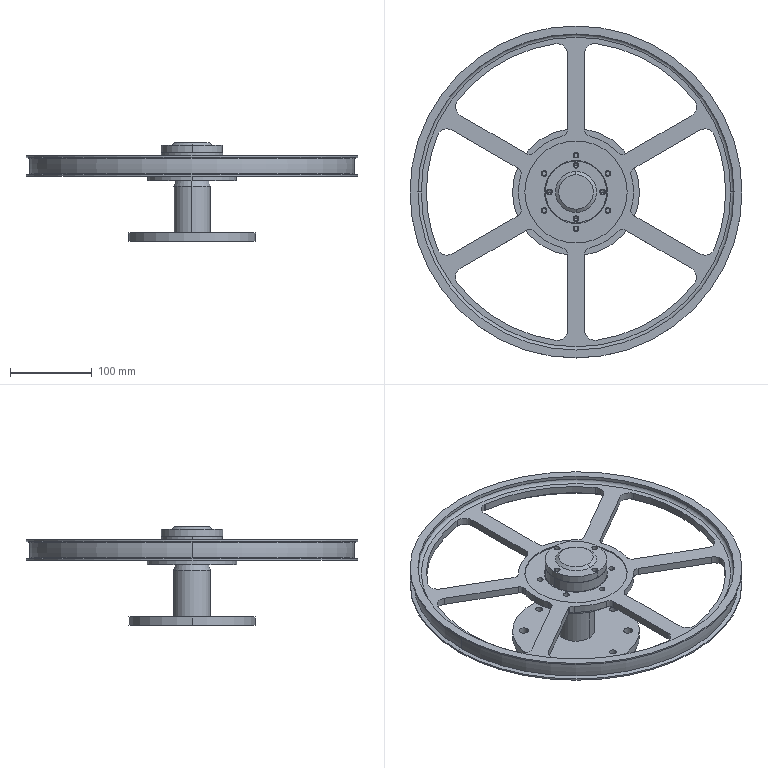Part | SolidWorks | 12 solids | 708 faces | box 405 x 405 x 120 mm | volume 1021210 mm3 | cylinder 312 | sphere 132 | plane 116 | torus 100 | cone 48 | commonest cylinder face diameters 0.4 x40 5 x36 1.57 x24 7 x20 15 x18 25 x16